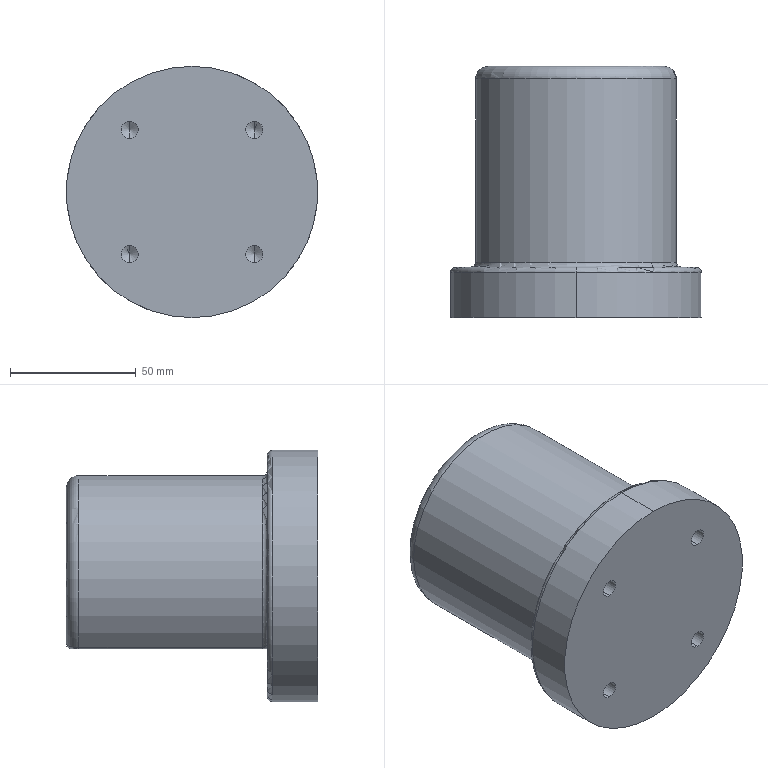Part | STEP file | Tube-changer group fixed foot SGN-2-14 | 1 solid | 39 faces | box 100 x 100 x 100 mm | volume 486001 mm3 | cylinder 16 | cone 8 | plane 7 | torus 4 | spline 4 | commonest cylinder face diameters 6.8 x8 4 x3 40 x2 100 x2 80 x1